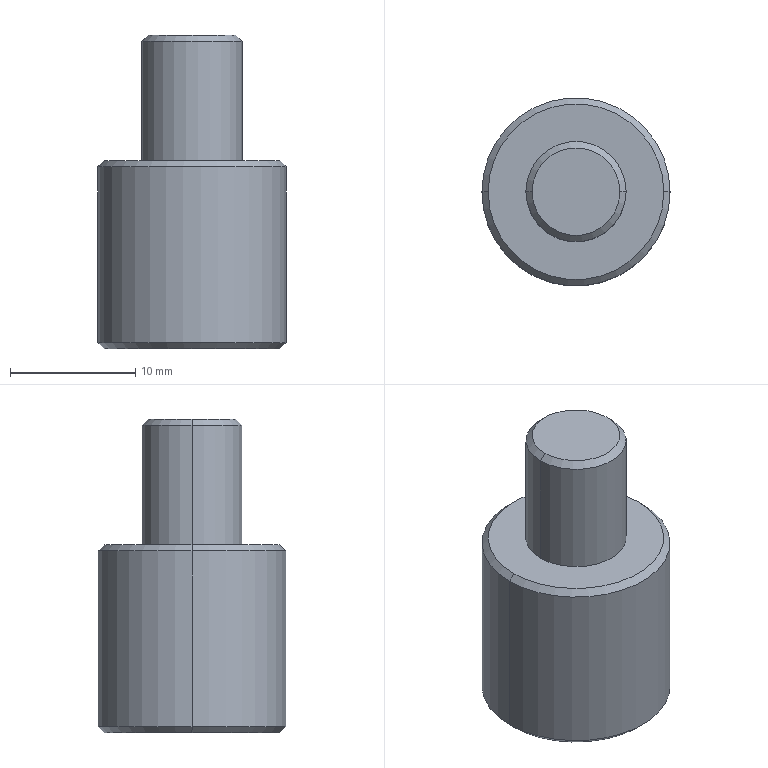Part | SolidWorks | features Chamfer 1, Extrusion 1, ICE 1 | 1 solid | 13 faces | box 15 x 15 x 25 mm | volume 3139 mm3 | cone 6 | cylinder 4 | plane 3 | commonest cylinder face diameters 8 x2 15 x2
STEP:
#1=CARTESIAN_POINT('',(3.5,0.,25.));
#2=VERTEX_POINT('',#1);
#3=CARTESIAN_POINT('',(-3.5,0.,25.));
#4=VERTEX_POINT('',#3);
#5=CARTESIAN_POINT('',(0.,0.,25.));
#6=DIRECTION('',(0.,0.,1.));
#7=DIRECTION('',(1.,0.,0.));
#8=AXIS2_PLACEMENT_3D('',#5,#6,#7);
#9=CIRCLE('',#8,3.5);
#10=EDGE_CURVE('',#2,#4,#9,.T.);
#11=ORIENTED_EDGE('',*,*,#10,.F.);
#12=CARTESIAN_POINT('',(4.,0.,24.5));
#13=VERTEX_POINT('',#12);
#14=CARTESIAN_POINT('',(3.5,0.,25.));
#15=DIRECTION('',(0.7071,0.,-0.7071));
#16=VECTOR('',#15,1000.);
#17=LINE('',#14,#16);
#18=EDGE_CURVE('',#2,#13,#17,.T.);
#19=ORIENTED_EDGE('',*,*,#18,.T.);
#20=CARTESIAN_POINT('',(-4.,0.,24.5));
#21=VERTEX_POINT('',#20);
#22=CARTESIAN_POINT('',(0.,0.,24.5));
#23=DIRECTION('',(0.,0.,-1.));
#24=DIRECTION('',(1.,0.,0.));
#25=AXIS2_PLACEMENT_3D('',#22,#23,#24);
#26=CIRCLE('',#25,4.);
#27=EDGE_CURVE('',#21,#13,#26,.T.);
#28=ORIENTED_EDGE('',*,*,#27,.F.);
#29=CARTESIAN_POINT('',(-3.5,0.,25.));
#30=DIRECTION('',(-0.7071,0.,-0.7071));
#31=VECTOR('',#30,1000.);
#32=LINE('',#29,#31);
#33=EDGE_CURVE('',#4,#21,#32,.T.);
#34=ORIENTED_EDGE('',*,*,#33,.F.);
#35=EDGE_LOOP('',(#11,#19,#28,#34));
#36=FACE_OUTER_BOUND('',#35,.T.);
#37=CARTESIAN_POINT('',(0.,0.,25.));
#38=DIRECTION('',(0.,0.,-1.));
#39=DIRECTION('',(-1.,0.,0.));
#40=AXIS2_PLACEMENT_3D('',#37,#38,#39);
#41=CONICAL_SURFACE('',#40,3.5,0.7854);
#42=ADVANCED_FACE('',(#36),#41,.T.);
#43=CARTESIAN_POINT('',(7.,0.,15.));
#44=VERTEX_POINT('',#43);
#45=CARTESIAN_POINT('',(-7.,0.,15.));
#46=VERTEX_POINT('',#45);
#47=CARTESIAN_POINT('',(0.,0.,15.));
#48=DIRECTION('',(0.,0.,1.));
#49=DIRECTION('',(1.,0.,0.));
#50=AXIS2_PLACEMENT_3D('',#47,#48,#49);
#51=CIRCLE('',#50,7.);
#52=EDGE_CURVE('',#44,#46,#51,.T.);
#53=ORIENTED_EDGE('',*,*,#52,.F.);
#54=CARTESIAN_POINT('',(7.5,0.,14.5));
#55=VERTEX_POINT('',#54);
#56=CARTESIAN_POINT('',(7.,0.,15.));
#57=DIRECTION('',(0.7071,0.,-0.7071));
#58=VECTOR('',#57,1000.);
#59=LINE('',#56,#58);
#60=EDGE_CURVE('',#44,#55,#59,.T.);
#61=ORIENTED_EDGE('',*,*,#60,.T.);
#62=CARTESIAN_POINT('',(-7.5,0.,14.5));
#63=VERTEX_POINT('',#62);
#64=CARTESIAN_POINT('',(0.,0.,14.5));
#65=DIRECTION('',(0.,0.,-1.));
#66=DIRECTION('',(1.,0.,0.));
#67=AXIS2_PLACEMENT_3D('',#64,#65,#66);
#68=CIRCLE('',#67,7.5);
#69=EDGE_CURVE('',#63,#55,#68,.T.);
#70=ORIENTED_EDGE('',*,*,#69,.F.);
#71=CARTESIAN_POINT('',(-7.,0.,15.));
#72=DIRECTION('',(-0.7071,0.,-0.7071));
#73=VECTOR('',#72,1000.);
#74=LINE('',#71,#73);
#75=EDGE_CURVE('',#46,#63,#74,.T.);
#76=ORIENTED_EDGE('',*,*,#75,.F.);
#77=EDGE_LOOP('',(#53,#61,#70,#76));
#78=FACE_OUTER_BOUND('',#77,.T.);
#79=CARTESIAN_POINT('',(0.,0.,15.));
#80=DIRECTION('',(0.,0.,-1.));
#81=DIRECTION('',(-1.,0.,0.));
#82=AXIS2_PLACEMENT_3D('',#79,#80,#81);
#83=CONICAL_SURFACE('',#82,7.,0.7854);
#84=ADVANCED_FACE('',(#78),#83,.T.);
#85=CARTESIAN_POINT('',(-7.,0.,0.));
#86=VERTEX_POINT('',#85);
#87=CARTESIAN_POINT('',(7.,0.,0.));
#88=VERTEX_POINT('',#87);
#89=CARTESIAN_POINT('',(0.,0.,0.));
#90=DIRECTION('',(0.,0.,-1.));
#91=DIRECTION('',(1.,0.,0.));
#92=AXIS2_PLACEMENT_3D('',#89,#90,#91);
#93=CIRCLE('',#92,7.);
#94=EDGE_CURVE('',#86,#88,#93,.T.);
#95=ORIENTED_EDGE('',*,*,#94,.F.);
#96=CARTESIAN_POINT('',(-7.5,0.,0.5));
#97=VERTEX_POINT('',#96);
#98=CARTESIAN_POINT('',(-7.5,0.,0.5));
#99=DIRECTION('',(-0.7071,0.,0.7071));
#100=VECTOR('',#99,1000.);
#101=LINE('',#98,#100);
#102=EDGE_CURVE('',#86,#97,#101,.T.);
#103=ORIENTED_EDGE('',*,*,#102,.T.);
#104=CARTESIAN_POINT('',(7.5,0.,0.5));
#105=VERTEX_POINT('',#104);
#106=CARTESIAN_POINT('',(0.,0.,0.5));
#107=DIRECTION('',(0.,0.,1.));
#108=DIRECTION('',(1.,0.,0.));
#109=AXIS2_PLACEMENT_3D('',#106,#107,#108);
#110=CIRCLE('',#109,7.5);
#111=EDGE_CURVE('',#105,#97,#110,.T.);
#112=ORIENTED_EDGE('',*,*,#111,.F.);
#113=CARTESIAN_POINT('',(7.5,0.,0.5));
#114=DIRECTION('',(0.7071,0.,0.7071));
#115=VECTOR('',#114,1000.);
#116=LINE('',#113,#115);
#117=EDGE_CURVE('',#88,#105,#116,.T.);
#118=ORIENTED_EDGE('',*,*,#117,.F.);
#119=EDGE_LOOP('',(#95,#103,#112,#118));
#120=FACE_OUTER_BOUND('',#119,.T.);
#121=CARTESIAN_POINT('',(0.,0.,0.5));
#122=DIRECTION('',(0.,0.,1.));
#123=DIRECTION('',(1.,0.,0.));
#124=AXIS2_PLACEMENT_3D('',#121,#122,#123);
#125=CONICAL_SURFACE('',#124,7.5,0.7854);
#126=ADVANCED_FACE('',(#120),#125,.T.);
#127=ORIENTED_EDGE('',*,*,#27,.T.);
#128=CARTESIAN_POINT('',(4.,0.,15.));
#129=VERTEX_POINT('',#128);
#130=CARTESIAN_POINT('',(4.,0.,25.));
#131=DIRECTION('',(0.,0.,-1.));
#132=VECTOR('',#131,1000.);
#133=LINE('',#130,#132);
#134=EDGE_CURVE('',#13,#129,#133,.T.);
#135=ORIENTED_EDGE('',*,*,#134,.T.);
#136=CARTESIAN_POINT('',(-4.,0.,15.));
#137=VERTEX_POINT('',#136);
#138=CARTESIAN_POINT('',(0.,0.,15.));
#139=DIRECTION('',(0.,0.,1.));
#140=DIRECTION('',(1.,0.,0.));
#141=AXIS2_PLACEMENT_3D('',#138,#139,#140);
#142=CIRCLE('',#141,4.);
#143=EDGE_CURVE('',#129,#137,#142,.T.);
#144=ORIENTED_EDGE('',*,*,#143,.T.);
#145=CARTESIAN_POINT('',(-4.,0.,25.));
#146=DIRECTION('',(0.,0.,-1.));
#147=VECTOR('',#146,1000.);
#148=LINE('',#145,#147);
#149=EDGE_CURVE('',#21,#137,#148,.T.);
#150=ORIENTED_EDGE('',*,*,#149,.F.);
#151=EDGE_LOOP('',(#127,#135,#144,#150));
#152=FACE_OUTER_BOUND('',#151,.T.);
#153=CARTESIAN_POINT('',(0.,0.,25.));
#154=DIRECTION('',(0.,0.,-1.));
#155=DIRECTION('',(-1.,0.,0.));
#156=AXIS2_PLACEMENT_3D('',#153,#154,#155);
#157=CYLINDRICAL_SURFACE('',#156,4.);
#158=ADVANCED_FACE('',(#152),#157,.T.);
#159=ORIENTED_EDGE('',*,*,#69,.T.);
#160=CARTESIAN_POINT('',(7.5,0.,15.));
#161=DIRECTION('',(0.,0.,-1.));
#162=VECTOR('',#161,1000.);
#163=LINE('',#160,#162);
#164=EDGE_CURVE('',#55,#105,#163,.T.);
#165=ORIENTED_EDGE('',*,*,#164,.T.);
#166=ORIENTED_EDGE('',*,*,#111,.T.);
#167=CARTESIAN_POINT('',(-7.5,0.,15.));
#168=DIRECTION('',(0.,0.,-1.));
#169=VECTOR('',#168,1000.);
#170=LINE('',#167,#169);
#171=EDGE_CURVE('',#63,#97,#170,.T.);
#172=ORIENTED_EDGE('',*,*,#171,.F.);
#173=EDGE_LOOP('',(#159,#165,#166,#172));
#174=FACE_OUTER_BOUND('',#173,.T.);
#175=CARTESIAN_POINT('',(0.,0.,15.));
#176=DIRECTION('',(0.,0.,-1.));
#177=DIRECTION('',(-1.,0.,0.));
#178=AXIS2_PLACEMENT_3D('',#175,#176,#177);
#179=CYLINDRICAL_SURFACE('',#178,7.5);
#180=ADVANCED_FACE('',(#174),#179,.T.);
#181=CARTESIAN_POINT('',(0.,0.,15.));
#182=DIRECTION('',(0.,0.,1.));
#183=DIRECTION('',(1.,0.,0.));
#184=AXIS2_PLACEMENT_3D('',#181,#182,#183);
#185=CIRCLE('',#184,7.);
#186=EDGE_CURVE('',#46,#44,#185,.T.);
#187=ORIENTED_EDGE('',*,*,#186,.T.);
#188=ORIENTED_EDGE('',*,*,#52,.T.);
#189=EDGE_LOOP('',(#187,#188));
#190=FACE_OUTER_BOUND('',#189,.T.);
#191=CARTESIAN_POINT('',(0.,0.,15.));
#192=DIRECTION('',(0.,0.,1.));
#193=DIRECTION('',(1.,0.,0.));
#194=AXIS2_PLACEMENT_3D('',#191,#192,#193);
#195=CIRCLE('',#194,4.);
#196=EDGE_CURVE('',#137,#129,#195,.T.);
#197=ORIENTED_EDGE('',*,*,#196,.F.);
#198=ORIENTED_EDGE('',*,*,#143,.F.);
#199=EDGE_LOOP('',(#197,#198));
#200=FACE_BOUND('',#199,.T.);
#201=CARTESIAN_POINT('',(0.,0.,15.));
#202=DIRECTION('',(0.,0.,1.));
#203=DIRECTION('',(1.,0.,0.));
#204=AXIS2_PLACEMENT_3D('',#201,#202,#203);
#205=PLANE('',#204);
#206=ADVANCED_FACE('',(#190,#200),#205,.T.);
#207=ORIENTED_EDGE('',*,*,#164,.F.);
#208=CARTESIAN_POINT('',(0.,0.,14.5));
#209=DIRECTION('',(0.,0.,-1.));
#210=DIRECTION('',(1.,0.,0.));
#211=AXIS2_PLACEMENT_3D('',#208,#209,#210);
#212=CIRCLE('',#211,7.5);
#213=EDGE_CURVE('',#55,#63,#212,.T.);
#214=ORIENTED_EDGE('',*,*,#213,.T.);
#215=ORIENTED_EDGE('',*,*,#171,.T.);
#216=CARTESIAN_POINT('',(0.,0.,0.5));
#217=DIRECTION('',(0.,0.,1.));
#218=DIRECTION('',(1.,0.,0.));
#219=AXIS2_PLACEMENT_3D('',#216,#217,#218);
#220=CIRCLE('',#219,7.5);
#221=EDGE_CURVE('',#97,#105,#220,.T.);
#222=ORIENTED_EDGE('',*,*,#221,.T.);
#223=EDGE_LOOP('',(#207,#214,#215,#222));
#224=FACE_OUTER_BOUND('',#223,.T.);
#225=CARTESIAN_POINT('',(0.,0.,15.));
#226=DIRECTION('',(0.,0.,-1.));
#227=DIRECTION('',(-1.,0.,0.));
#228=AXIS2_PLACEMENT_3D('',#225,#226,#227);
#229=CYLINDRICAL_SURFACE('',#228,7.5);
#230=ADVANCED_FACE('',(#224),#229,.T.);
#231=CARTESIAN_POINT('',(0.,0.,0.));
#232=DIRECTION('',(0.,0.,-1.));
#233=DIRECTION('',(1.,0.,0.));
#234=AXIS2_PLACEMENT_3D('',#231,#232,#233);
#235=CIRCLE('',#234,7.);
#236=EDGE_CURVE('',#88,#86,#235,.T.);
#237=ORIENTED_EDGE('',*,*,#236,.T.);
#238=ORIENTED_EDGE('',*,*,#94,.T.);
#239=EDGE_LOOP('',(#237,#238));
#240=FACE_OUTER_BOUND('',#239,.T.);
#241=CARTESIAN_POINT('',(0.,0.,0.));
#242=DIRECTION('',(0.,0.,1.));
#243=DIRECTION('',(1.,0.,0.));
#244=AXIS2_PLACEMENT_3D('',#241,#242,#243);
#245=PLANE('',#244);
#246=ADVANCED_FACE('',(#240),#245,.F.);
#247=ORIENTED_EDGE('',*,*,#134,.F.);
#248=CARTESIAN_POINT('',(0.,0.,24.5));
#249=DIRECTION('',(0.,0.,-1.));
#250=DIRECTION('',(1.,0.,0.));
#251=AXIS2_PLACEMENT_3D('',#248,#249,#250);
#252=CIRCLE('',#251,4.);
#253=EDGE_CURVE('',#13,#21,#252,.T.);
#254=ORIENTED_EDGE('',*,*,#253,.T.);
#255=ORIENTED_EDGE('',*,*,#149,.T.);
#256=ORIENTED_EDGE('',*,*,#196,.T.);
#257=EDGE_LOOP('',(#247,#254,#255,#256));
#258=FACE_OUTER_BOUND('',#257,.T.);
#259=CARTESIAN_POINT('',(0.,0.,25.));
#260=DIRECTION('',(0.,0.,-1.));
#261=DIRECTION('',(-1.,0.,0.));
#262=AXIS2_PLACEMENT_3D('',#259,#260,#261);
#263=CYLINDRICAL_SURFACE('',#262,4.);
#264=ADVANCED_FACE('',(#258),#263,.T.);
#265=CARTESIAN_POINT('',(0.,0.,25.));
#266=DIRECTION('',(0.,0.,1.));
#267=DIRECTION('',(1.,0.,0.));
#268=AXIS2_PLACEMENT_3D('',#265,#266,#267);
#269=CIRCLE('',#268,3.5);
#270=EDGE_CURVE('',#4,#2,#269,.T.);
#271=ORIENTED_EDGE('',*,*,#270,.T.);
#272=ORIENTED_EDGE('',*,*,#10,.T.);
#273=EDGE_LOOP('',(#271,#272));
#274=FACE_OUTER_BOUND('',#273,.T.);
#275=CARTESIAN_POINT('',(0.,0.,25.));
#276=DIRECTION('',(0.,0.,1.));
#277=DIRECTION('',(1.,0.,0.));
#278=AXIS2_PLACEMENT_3D('',#275,#276,#277);
#279=PLANE('',#278);
#280=ADVANCED_FACE('',(#274),#279,.T.);
#281=ORIENTED_EDGE('',*,*,#102,.F.);
#282=ORIENTED_EDGE('',*,*,#236,.F.);
#283=ORIENTED_EDGE('',*,*,#117,.T.);
#284=ORIENTED_EDGE('',*,*,#221,.F.);
#285=EDGE_LOOP('',(#281,#282,#283,#284));
#286=FACE_OUTER_BOUND('',#285,.T.);
#287=CARTESIAN_POINT('',(0.,0.,0.5));
#288=DIRECTION('',(0.,0.,1.));
#289=DIRECTION('',(1.,0.,0.));
#290=AXIS2_PLACEMENT_3D('',#287,#288,#289);
#291=CONICAL_SURFACE('',#290,7.5,0.7854);
#292=ADVANCED_FACE('',(#286),#291,.T.);
#293=ORIENTED_EDGE('',*,*,#60,.F.);
#294=ORIENTED_EDGE('',*,*,#186,.F.);
#295=ORIENTED_EDGE('',*,*,#75,.T.);
#296=ORIENTED_EDGE('',*,*,#213,.F.);
#297=EDGE_LOOP('',(#293,#294,#295,#296));
#298=FACE_OUTER_BOUND('',#297,.T.);
#299=CARTESIAN_POINT('',(0.,0.,15.));
#300=DIRECTION('',(0.,0.,-1.));
#301=DIRECTION('',(-1.,0.,0.));
#302=AXIS2_PLACEMENT_3D('',#299,#300,#301);
#303=CONICAL_SURFACE('',#302,7.,0.7854);
#304=ADVANCED_FACE('',(#298),#303,.T.);
#305=ORIENTED_EDGE('',*,*,#18,.F.);
#306=ORIENTED_EDGE('',*,*,#270,.F.);
#307=ORIENTED_EDGE('',*,*,#33,.T.);
#308=ORIENTED_EDGE('',*,*,#253,.F.);
#309=EDGE_LOOP('',(#305,#306,#307,#308));
#310=FACE_OUTER_BOUND('',#309,.T.);
#311=CARTESIAN_POINT('',(0.,0.,25.));
#312=DIRECTION('',(0.,0.,-1.));
#313=DIRECTION('',(-1.,0.,0.));
#314=AXIS2_PLACEMENT_3D('',#311,#312,#313);
#315=CONICAL_SURFACE('',#314,3.5,0.7854);
#316=ADVANCED_FACE('',(#310),#315,.T.);
#317=CLOSED_SHELL('',(#42,#84,#126,#158,#180,#206,#230,#246,#264,#280,#292,#304,#316));
#318=MANIFOLD_SOLID_BREP('',#317);
#319=CARTESIAN_POINT('',(0.,0.,0.));
#320=DIRECTION('',(0.,0.,1.));
#321=DIRECTION('',(1.,0.,0.));
#322=AXIS2_PLACEMENT_3D('',#319,#320,#321);
#323=(LENGTH_UNIT()NAMED_UNIT(*)SI_UNIT(.MILLI.,.METRE.));
#324=UNCERTAINTY_MEASURE_WITH_UNIT(LENGTH_MEASURE(0.00001),#323,'','');
#325=(NAMED_UNIT(*)PLANE_ANGLE_UNIT()SI_UNIT($,.RADIAN.));
#326=(NAMED_UNIT(*)SI_UNIT($,.STERADIAN.)SOLID_ANGLE_UNIT());
#327=(GEOMETRIC_REPRESENTATION_CONTEXT(3)GLOBAL_UNCERTAINTY_ASSIGNED_CONTEXT((#324))GLOBAL_UNIT_ASSIGNED_CONTEXT((#323,#325,#326))REPRESENTATION_CONTEXT('',''));
#328=ADVANCED_BREP_SHAPE_REPRESENTATION('',(#318,#322),#327);